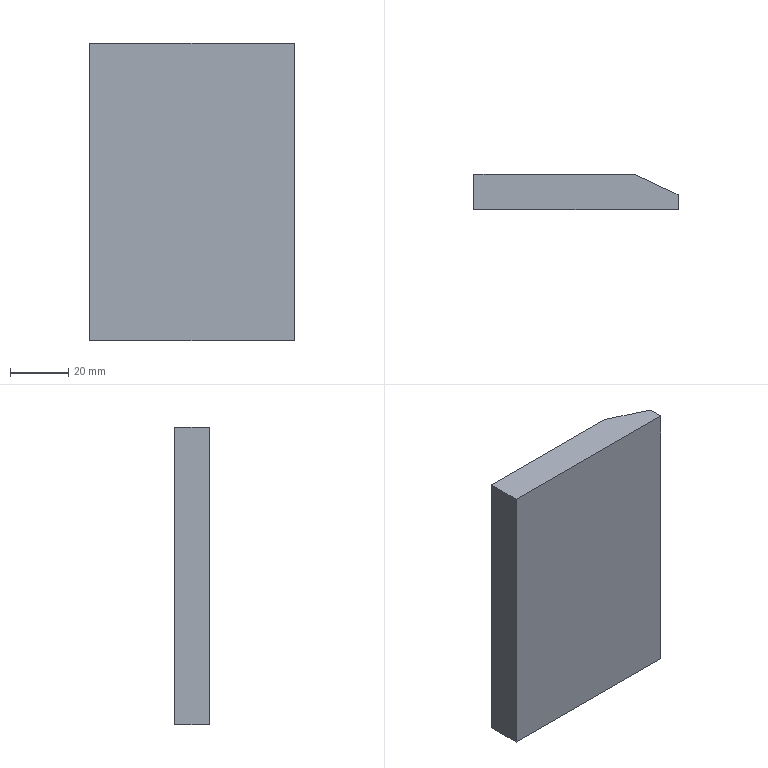Part | SolidWorks | features Extrusion 1 | 1 solid | 7 faces | box 70 x 12 x 102 mm | volume 80325 mm3 | plane 7
STEP:
#1=CARTESIAN_POINT('',(-70.,0.,0.));
#2=VERTEX_POINT('',#1);
#3=CARTESIAN_POINT('',(0.,0.,0.));
#4=VERTEX_POINT('',#3);
#5=CARTESIAN_POINT('',(-70.,0.,0.));
#6=DIRECTION('',(1.,0.,0.));
#7=VECTOR('',#6,1000.);
#8=LINE('',#5,#7);
#9=EDGE_CURVE('',#2,#4,#8,.T.);
#10=ORIENTED_EDGE('',*,*,#9,.T.);
#11=CARTESIAN_POINT('',(0.,0.,102.));
#12=VERTEX_POINT('',#11);
#13=CARTESIAN_POINT('',(0.,0.,102.));
#14=DIRECTION('',(0.,0.,-1.));
#15=VECTOR('',#14,1000.);
#16=LINE('',#13,#15);
#17=EDGE_CURVE('',#12,#4,#16,.T.);
#18=ORIENTED_EDGE('',*,*,#17,.F.);
#19=CARTESIAN_POINT('',(-70.,0.,102.));
#20=VERTEX_POINT('',#19);
#21=CARTESIAN_POINT('',(-70.,0.,102.));
#22=DIRECTION('',(1.,0.,0.));
#23=VECTOR('',#22,1000.);
#24=LINE('',#21,#23);
#25=EDGE_CURVE('',#20,#12,#24,.T.);
#26=ORIENTED_EDGE('',*,*,#25,.F.);
#27=CARTESIAN_POINT('',(-70.,0.,102.));
#28=DIRECTION('',(0.,0.,-1.));
#29=VECTOR('',#28,1000.);
#30=LINE('',#27,#29);
#31=EDGE_CURVE('',#20,#2,#30,.T.);
#32=ORIENTED_EDGE('',*,*,#31,.T.);
#33=EDGE_LOOP('',(#10,#18,#26,#32));
#34=FACE_OUTER_BOUND('',#33,.T.);
#35=CARTESIAN_POINT('',(-70.,0.,102.));
#36=DIRECTION('',(0.,1.,0.));
#37=DIRECTION('',(0.,0.,1.));
#38=AXIS2_PLACEMENT_3D('',#35,#36,#37);
#39=PLANE('',#38);
#40=ADVANCED_FACE('',(#34),#39,.F.);
#41=CARTESIAN_POINT('',(0.,5.,0.));
#42=VERTEX_POINT('',#41);
#43=CARTESIAN_POINT('',(0.,0.,0.));
#44=DIRECTION('',(0.,1.,0.));
#45=VECTOR('',#44,1000.);
#46=LINE('',#43,#45);
#47=EDGE_CURVE('',#4,#42,#46,.T.);
#48=ORIENTED_EDGE('',*,*,#47,.T.);
#49=CARTESIAN_POINT('',(0.,5.,102.));
#50=VERTEX_POINT('',#49);
#51=CARTESIAN_POINT('',(0.,5.,102.));
#52=DIRECTION('',(0.,0.,-1.));
#53=VECTOR('',#52,1000.);
#54=LINE('',#51,#53);
#55=EDGE_CURVE('',#50,#42,#54,.T.);
#56=ORIENTED_EDGE('',*,*,#55,.F.);
#57=CARTESIAN_POINT('',(0.,0.,102.));
#58=DIRECTION('',(0.,1.,0.));
#59=VECTOR('',#58,1000.);
#60=LINE('',#57,#59);
#61=EDGE_CURVE('',#12,#50,#60,.T.);
#62=ORIENTED_EDGE('',*,*,#61,.F.);
#63=ORIENTED_EDGE('',*,*,#17,.T.);
#64=EDGE_LOOP('',(#48,#56,#62,#63));
#65=FACE_OUTER_BOUND('',#64,.T.);
#66=CARTESIAN_POINT('',(0.,0.,102.));
#67=DIRECTION('',(-1.,0.,0.));
#68=DIRECTION('',(0.,0.,1.));
#69=AXIS2_PLACEMENT_3D('',#66,#67,#68);
#70=PLANE('',#69);
#71=ADVANCED_FACE('',(#65),#70,.F.);
#72=CARTESIAN_POINT('',(-15.,12.,0.));
#73=VERTEX_POINT('',#72);
#74=CARTESIAN_POINT('',(0.,5.,0.));
#75=DIRECTION('',(-0.9062,0.4229,0.));
#76=VECTOR('',#75,1000.);
#77=LINE('',#74,#76);
#78=EDGE_CURVE('',#42,#73,#77,.T.);
#79=ORIENTED_EDGE('',*,*,#78,.T.);
#80=CARTESIAN_POINT('',(-15.,12.,102.));
#81=VERTEX_POINT('',#80);
#82=CARTESIAN_POINT('',(-15.,12.,102.));
#83=DIRECTION('',(0.,0.,-1.));
#84=VECTOR('',#83,1000.);
#85=LINE('',#82,#84);
#86=EDGE_CURVE('',#81,#73,#85,.T.);
#87=ORIENTED_EDGE('',*,*,#86,.F.);
#88=CARTESIAN_POINT('',(0.,5.,102.));
#89=DIRECTION('',(-0.9062,0.4229,0.));
#90=VECTOR('',#89,1000.);
#91=LINE('',#88,#90);
#92=EDGE_CURVE('',#50,#81,#91,.T.);
#93=ORIENTED_EDGE('',*,*,#92,.F.);
#94=ORIENTED_EDGE('',*,*,#55,.T.);
#95=EDGE_LOOP('',(#79,#87,#93,#94));
#96=FACE_OUTER_BOUND('',#95,.T.);
#97=CARTESIAN_POINT('',(0.,5.,102.));
#98=DIRECTION('',(-0.4229,-0.9062,0.));
#99=DIRECTION('',(0.9062,-0.4229,0.));
#100=AXIS2_PLACEMENT_3D('',#97,#98,#99);
#101=PLANE('',#100);
#102=ADVANCED_FACE('',(#96),#101,.F.);
#103=CARTESIAN_POINT('',(-70.,12.,0.));
#104=VERTEX_POINT('',#103);
#105=CARTESIAN_POINT('',(-15.,12.,0.));
#106=DIRECTION('',(-1.,0.,0.));
#107=VECTOR('',#106,1000.);
#108=LINE('',#105,#107);
#109=EDGE_CURVE('',#73,#104,#108,.T.);
#110=ORIENTED_EDGE('',*,*,#109,.T.);
#111=CARTESIAN_POINT('',(-70.,12.,102.));
#112=VERTEX_POINT('',#111);
#113=CARTESIAN_POINT('',(-70.,12.,102.));
#114=DIRECTION('',(0.,0.,-1.));
#115=VECTOR('',#114,1000.);
#116=LINE('',#113,#115);
#117=EDGE_CURVE('',#112,#104,#116,.T.);
#118=ORIENTED_EDGE('',*,*,#117,.F.);
#119=CARTESIAN_POINT('',(-15.,12.,102.));
#120=DIRECTION('',(-1.,0.,0.));
#121=VECTOR('',#120,1000.);
#122=LINE('',#119,#121);
#123=EDGE_CURVE('',#81,#112,#122,.T.);
#124=ORIENTED_EDGE('',*,*,#123,.F.);
#125=ORIENTED_EDGE('',*,*,#86,.T.);
#126=EDGE_LOOP('',(#110,#118,#124,#125));
#127=FACE_OUTER_BOUND('',#126,.T.);
#128=CARTESIAN_POINT('',(-15.,12.,102.));
#129=DIRECTION('',(0.,-1.,0.));
#130=DIRECTION('',(1.,0.,0.));
#131=AXIS2_PLACEMENT_3D('',#128,#129,#130);
#132=PLANE('',#131);
#133=ADVANCED_FACE('',(#127),#132,.F.);
#134=CARTESIAN_POINT('',(-70.,0.,0.));
#135=DIRECTION('',(0.,-1.,0.));
#136=VECTOR('',#135,1000.);
#137=LINE('',#134,#136);
#138=EDGE_CURVE('',#104,#2,#137,.T.);
#139=ORIENTED_EDGE('',*,*,#138,.T.);
#140=ORIENTED_EDGE('',*,*,#31,.F.);
#141=CARTESIAN_POINT('',(-70.,0.,102.));
#142=DIRECTION('',(0.,-1.,0.));
#143=VECTOR('',#142,1000.);
#144=LINE('',#141,#143);
#145=EDGE_CURVE('',#112,#20,#144,.T.);
#146=ORIENTED_EDGE('',*,*,#145,.F.);
#147=ORIENTED_EDGE('',*,*,#117,.T.);
#148=EDGE_LOOP('',(#139,#140,#146,#147));
#149=FACE_OUTER_BOUND('',#148,.T.);
#150=CARTESIAN_POINT('',(-70.,0.,102.));
#151=DIRECTION('',(1.,0.,0.));
#152=DIRECTION('',(0.,0.,-1.));
#153=AXIS2_PLACEMENT_3D('',#150,#151,#152);
#154=PLANE('',#153);
#155=ADVANCED_FACE('',(#149),#154,.F.);
#156=ORIENTED_EDGE('',*,*,#25,.T.);
#157=ORIENTED_EDGE('',*,*,#61,.T.);
#158=ORIENTED_EDGE('',*,*,#92,.T.);
#159=ORIENTED_EDGE('',*,*,#123,.T.);
#160=ORIENTED_EDGE('',*,*,#145,.T.);
#161=EDGE_LOOP('',(#156,#157,#158,#159,#160));
#162=FACE_OUTER_BOUND('',#161,.T.);
#163=CARTESIAN_POINT('',(0.,0.,102.));
#164=DIRECTION('',(0.,0.,1.));
#165=DIRECTION('',(1.,0.,0.));
#166=AXIS2_PLACEMENT_3D('',#163,#164,#165);
#167=PLANE('',#166);
#168=ADVANCED_FACE('',(#162),#167,.T.);
#169=ORIENTED_EDGE('',*,*,#9,.F.);
#170=ORIENTED_EDGE('',*,*,#138,.F.);
#171=ORIENTED_EDGE('',*,*,#109,.F.);
#172=ORIENTED_EDGE('',*,*,#78,.F.);
#173=ORIENTED_EDGE('',*,*,#47,.F.);
#174=EDGE_LOOP('',(#169,#170,#171,#172,#173));
#175=FACE_OUTER_BOUND('',#174,.T.);
#176=CARTESIAN_POINT('',(0.,0.,0.));
#177=DIRECTION('',(0.,0.,1.));
#178=DIRECTION('',(1.,0.,0.));
#179=AXIS2_PLACEMENT_3D('',#176,#177,#178);
#180=PLANE('',#179);
#181=ADVANCED_FACE('',(#175),#180,.F.);
#182=CLOSED_SHELL('',(#40,#71,#102,#133,#155,#168,#181));
#183=MANIFOLD_SOLID_BREP('',#182);
#184=CARTESIAN_POINT('',(0.,0.,0.));
#185=DIRECTION('',(0.,0.,1.));
#186=DIRECTION('',(1.,0.,0.));
#187=AXIS2_PLACEMENT_3D('',#184,#185,#186);
#188=(LENGTH_UNIT()NAMED_UNIT(*)SI_UNIT(.MILLI.,.METRE.));
#189=UNCERTAINTY_MEASURE_WITH_UNIT(LENGTH_MEASURE(0.00001),#188,'','');
#190=(NAMED_UNIT(*)PLANE_ANGLE_UNIT()SI_UNIT($,.RADIAN.));
#191=(NAMED_UNIT(*)SI_UNIT($,.STERADIAN.)SOLID_ANGLE_UNIT());
#192=(GEOMETRIC_REPRESENTATION_CONTEXT(3)GLOBAL_UNCERTAINTY_ASSIGNED_CONTEXT((#189))GLOBAL_UNIT_ASSIGNED_CONTEXT((#188,#190,#191))REPRESENTATION_CONTEXT('',''));
#193=ADVANCED_BREP_SHAPE_REPRESENTATION('',(#183,#187),#192);